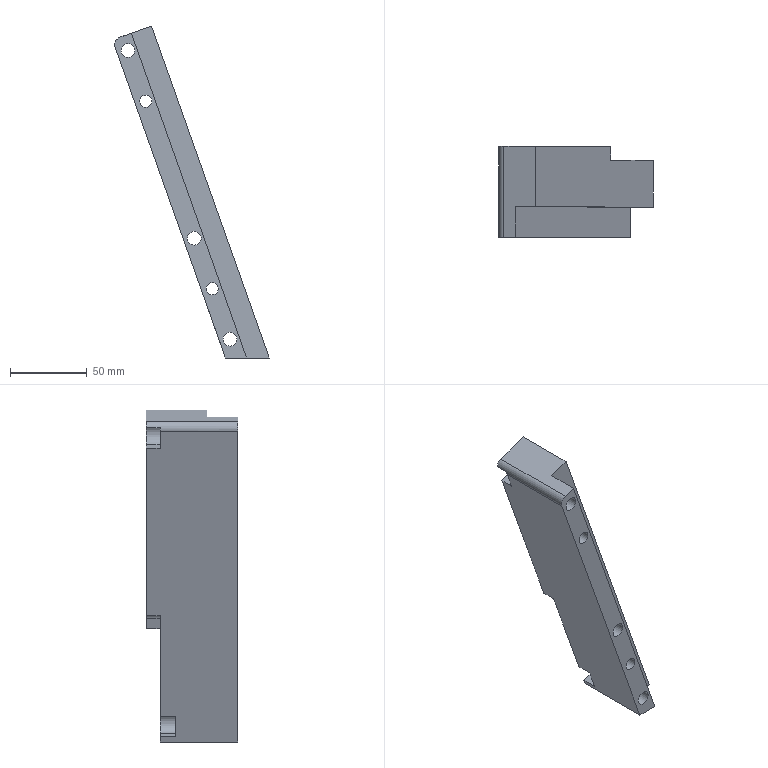Part | STEP file | SLIDE1-PLATE_id554_x_t | 1 solid | 27 faces | box 100.862 x 59.5 x 216.856 mm | volume 259316 mm3 | plane 18 | cylinder 9 | commonest cylinder face diameters 9 x3 14 x3 8 x2 10 x1
STEP:
#1=CARTESIAN_POINT('',(-1.05,-40.,-275.));
#2=VERTEX_POINT('',#1);
#3=CARTESIAN_POINT('',(13.802,-40.,-275.));
#4=VERTEX_POINT('',#3);
#5=CARTESIAN_POINT('',(-10.598,-40.,-275.));
#6=DIRECTION('',(1.,0.,0.));
#7=VECTOR('',#6,1.);
#8=LINE('',#5,#7);
#9=EDGE_CURVE('',#2,#4,#8,.T.);
#10=ORIENTED_EDGE('',*,*,#9,.T.);
#11=CARTESIAN_POINT('',(-62.991,-40.,-58.144));
#12=VERTEX_POINT('',#11);
#13=CARTESIAN_POINT('',(-62.991,-40.,-58.144));
#14=DIRECTION('',(0.3338,0.,-0.9426));
#15=VECTOR('',#14,1.);
#16=LINE('',#13,#15);
#17=EDGE_CURVE('',#12,#4,#16,.T.);
#18=ORIENTED_EDGE('',*,*,#17,.F.);
#19=CARTESIAN_POINT('',(-76.188,-40.,-62.818));
#20=VERTEX_POINT('',#19);
#21=CARTESIAN_POINT('',(11.277,-40.,-31.845));
#22=DIRECTION('',(-0.9426,0.,-0.3338));
#23=VECTOR('',#22,1.);
#24=LINE('',#21,#23);
#25=EDGE_CURVE('',#12,#20,#24,.T.);
#26=ORIENTED_EDGE('',*,*,#25,.T.);
#27=CARTESIAN_POINT('',(-76.188,-40.,-62.818));
#28=DIRECTION('',(0.3338,0.,-0.9426));
#29=VECTOR('',#28,1.);
#30=LINE('',#27,#29);
#31=EDGE_CURVE('',#20,#2,#30,.T.);
#32=ORIENTED_EDGE('',*,*,#31,.T.);
#33=EDGE_LOOP('',(#10,#18,#26,#32));
#34=FACE_OUTER_BOUND('',#33,.T.);
#35=CARTESIAN_POINT('',(-62.991,-40.,-58.144));
#36=DIRECTION('',(0.,1.,0.));
#37=DIRECTION('',(0.,0.,1.));
#38=AXIS2_PLACEMENT_3D('',#35,#36,#37);
#39=PLANE('',#38);
#40=ADVANCED_FACE('',(#34),#39,.F.);
#41=CARTESIAN_POINT('',(-1.05,-60.,-275.));
#42=VERTEX_POINT('',#41);
#43=CARTESIAN_POINT('',(-1.05,-0.5,-275.));
#44=DIRECTION('',(0.,1.,0.));
#45=VECTOR('',#44,1.);
#46=LINE('',#43,#45);
#47=EDGE_CURVE('',#42,#2,#46,.T.);
#48=ORIENTED_EDGE('',*,*,#47,.T.);
#49=ORIENTED_EDGE('',*,*,#31,.F.);
#50=CARTESIAN_POINT('',(-76.188,-60.,-62.818));
#51=VERTEX_POINT('',#50);
#52=CARTESIAN_POINT('',(-76.188,60.,-62.818));
#53=DIRECTION('',(0.,-1.,0.));
#54=VECTOR('',#53,1.);
#55=LINE('',#52,#54);
#56=EDGE_CURVE('',#20,#51,#55,.T.);
#57=ORIENTED_EDGE('',*,*,#56,.T.);
#58=CARTESIAN_POINT('',(-1.05,-60.,-275.));
#59=DIRECTION('',(-0.3338,0.,0.9426));
#60=VECTOR('',#59,1.);
#61=LINE('',#58,#60);
#62=EDGE_CURVE('',#42,#51,#61,.T.);
#63=ORIENTED_EDGE('',*,*,#62,.F.);
#64=EDGE_LOOP('',(#48,#49,#57,#63));
#65=FACE_OUTER_BOUND('',#64,.T.);
#66=CARTESIAN_POINT('',(-76.188,-40.,-62.818));
#67=DIRECTION('',(-0.9426,0.,-0.3338));
#68=DIRECTION('',(-0.3338,0.,0.9426));
#69=AXIS2_PLACEMENT_3D('',#66,#67,#68);
#70=PLANE('',#69);
#71=ADVANCED_FACE('',(#65),#70,.F.);
#72=CARTESIAN_POINT('',(-78.506,-60.,-69.747));
#73=VERTEX_POINT('',#72);
#74=CARTESIAN_POINT('',(-78.506,-60.,-74.247));
#75=DIRECTION('',(0.,1.,0.));
#76=DIRECTION('',(0.,0.,1.));
#77=AXIS2_PLACEMENT_3D('',#74,#75,#76);
#78=CIRCLE('',#77,4.5);
#79=EDGE_CURVE('',#73,#73,#78,.T.);
#80=ORIENTED_EDGE('',*,*,#79,.F.);
#81=EDGE_LOOP('',(#80));
#82=FACE_BOUND('',#81,.T.);
#83=CARTESIAN_POINT('',(-78.506,-9.5,-69.747));
#84=VERTEX_POINT('',#83);
#85=CARTESIAN_POINT('',(-78.506,-9.5,-74.247));
#86=DIRECTION('',(0.,-1.,0.));
#87=DIRECTION('',(0.,0.,1.));
#88=AXIS2_PLACEMENT_3D('',#85,#86,#87);
#89=CIRCLE('',#88,4.5);
#90=EDGE_CURVE('',#84,#84,#89,.T.);
#91=ORIENTED_EDGE('',*,*,#90,.F.);
#92=EDGE_LOOP('',(#91));
#93=FACE_BOUND('',#92,.T.);
#94=CARTESIAN_POINT('',(-78.506,-0.5,-74.247));
#95=DIRECTION('',(0.,1.,0.));
#96=DIRECTION('',(0.,0.,1.));
#97=AXIS2_PLACEMENT_3D('',#94,#95,#96);
#98=CYLINDRICAL_SURFACE('',#97,4.5);
#99=ADVANCED_FACE('',(#82,#93),#98,.F.);
#100=CARTESIAN_POINT('',(-80.842,-9.5,-67.648));
#101=VERTEX_POINT('',#100);
#102=CARTESIAN_POINT('',(-76.169,-9.5,-80.845));
#103=VERTEX_POINT('',#102);
#104=CARTESIAN_POINT('',(-78.506,-9.5,-74.247));
#105=DIRECTION('',(0.,1.,0.));
#106=DIRECTION('',(0.,0.,1.));
#107=AXIS2_PLACEMENT_3D('',#104,#105,#106);
#108=CIRCLE('',#107,7.);
#109=EDGE_CURVE('',#101,#103,#108,.T.);
#110=ORIENTED_EDGE('',*,*,#109,.F.);
#111=CARTESIAN_POINT('',(-80.842,-0.5,-67.648));
#112=VERTEX_POINT('',#111);
#113=CARTESIAN_POINT('',(-80.842,-0.5,-67.648));
#114=DIRECTION('',(0.,1.,0.));
#115=VECTOR('',#114,1.);
#116=LINE('',#113,#115);
#117=EDGE_CURVE('',#101,#112,#116,.T.);
#118=ORIENTED_EDGE('',*,*,#117,.T.);
#119=CARTESIAN_POINT('',(-76.169,-0.5,-80.845));
#120=VERTEX_POINT('',#119);
#121=CARTESIAN_POINT('',(-78.506,-0.5,-74.247));
#122=DIRECTION('',(0.,-1.,0.));
#123=DIRECTION('',(0.,0.,1.));
#124=AXIS2_PLACEMENT_3D('',#121,#122,#123);
#125=CIRCLE('',#124,7.);
#126=EDGE_CURVE('',#120,#112,#125,.T.);
#127=ORIENTED_EDGE('',*,*,#126,.F.);
#128=CARTESIAN_POINT('',(-76.169,-0.5,-80.845));
#129=DIRECTION('',(0.,-1.,0.));
#130=VECTOR('',#129,1.);
#131=LINE('',#128,#130);
#132=EDGE_CURVE('',#120,#103,#131,.T.);
#133=ORIENTED_EDGE('',*,*,#132,.T.);
#134=EDGE_LOOP('',(#110,#118,#127,#133));
#135=FACE_OUTER_BOUND('',#134,.T.);
#136=CARTESIAN_POINT('',(-78.506,-0.5,-74.247));
#137=DIRECTION('',(0.,1.,0.));
#138=DIRECTION('',(0.,0.,1.));
#139=AXIS2_PLACEMENT_3D('',#136,#137,#138);
#140=CYLINDRICAL_SURFACE('',#139,7.);
#141=ADVANCED_FACE('',(#135),#140,.F.);
#142=CARTESIAN_POINT('',(-87.047,-9.5,-69.846));
#143=VERTEX_POINT('',#142);
#144=CARTESIAN_POINT('',(-87.047,-9.5,-69.846));
#145=DIRECTION('',(0.9426,0.,0.3338));
#146=VECTOR('',#145,1.);
#147=LINE('',#144,#146);
#148=EDGE_CURVE('',#143,#101,#147,.T.);
#149=ORIENTED_EDGE('',*,*,#148,.F.);
#150=CARTESIAN_POINT('',(-87.047,-0.5,-69.846));
#151=VERTEX_POINT('',#150);
#152=CARTESIAN_POINT('',(-87.047,-0.5,-69.846));
#153=DIRECTION('',(0.,-1.,0.));
#154=VECTOR('',#153,1.);
#155=LINE('',#152,#154);
#156=EDGE_CURVE('',#151,#143,#155,.T.);
#157=ORIENTED_EDGE('',*,*,#156,.F.);
#158=CARTESIAN_POINT('',(-80.842,-0.5,-67.648));
#159=DIRECTION('',(-0.9426,0.,-0.3338));
#160=VECTOR('',#159,1.);
#161=LINE('',#158,#160);
#162=EDGE_CURVE('',#112,#151,#161,.T.);
#163=ORIENTED_EDGE('',*,*,#162,.F.);
#164=ORIENTED_EDGE('',*,*,#117,.F.);
#165=EDGE_LOOP('',(#149,#157,#163,#164));
#166=FACE_OUTER_BOUND('',#165,.T.);
#167=CARTESIAN_POINT('',(-94.861,-0.5,-72.613));
#168=DIRECTION('',(-0.3338,0.,0.9426));
#169=DIRECTION('',(0.9426,0.,0.3338));
#170=AXIS2_PLACEMENT_3D('',#167,#168,#169);
#171=PLANE('',#170);
#172=ADVANCED_FACE('',(#166),#171,.F.);
#173=CARTESIAN_POINT('',(-62.991,-0.5,-58.144));
#174=VERTEX_POINT('',#173);
#175=CARTESIAN_POINT('',(-62.991,-0.5,-58.144));
#176=DIRECTION('',(0.,-1.,0.));
#177=VECTOR('',#176,1.);
#178=LINE('',#175,#177);
#179=EDGE_CURVE('',#174,#12,#178,.T.);
#180=ORIENTED_EDGE('',*,*,#179,.F.);
#181=CARTESIAN_POINT('',(-83.729,-0.5,-65.488));
#182=VERTEX_POINT('',#181);
#183=CARTESIAN_POINT('',(-83.729,-0.5,-65.488));
#184=DIRECTION('',(0.9426,0.,0.3338));
#185=VECTOR('',#184,1.);
#186=LINE('',#183,#185);
#187=EDGE_CURVE('',#182,#174,#186,.T.);
#188=ORIENTED_EDGE('',*,*,#187,.F.);
#189=CARTESIAN_POINT('',(-83.729,-60.,-65.488));
#190=VERTEX_POINT('',#189);
#191=CARTESIAN_POINT('',(-83.729,-0.5,-65.488));
#192=DIRECTION('',(0.,1.,0.));
#193=VECTOR('',#192,1.);
#194=LINE('',#191,#193);
#195=EDGE_CURVE('',#190,#182,#194,.T.);
#196=ORIENTED_EDGE('',*,*,#195,.F.);
#197=CARTESIAN_POINT('',(-76.188,-60.,-62.818));
#198=DIRECTION('',(-0.9426,0.,-0.3338));
#199=VECTOR('',#198,1.);
#200=LINE('',#197,#199);
#201=EDGE_CURVE('',#51,#190,#200,.T.);
#202=ORIENTED_EDGE('',*,*,#201,.F.);
#203=ORIENTED_EDGE('',*,*,#56,.F.);
#204=ORIENTED_EDGE('',*,*,#25,.F.);
#205=EDGE_LOOP('',(#180,#188,#196,#202,#203,#204));
#206=FACE_OUTER_BOUND('',#205,.T.);
#207=CARTESIAN_POINT('',(11.277,60.,-31.845));
#208=DIRECTION('',(0.3338,0.,-0.9426));
#209=DIRECTION('',(-0.9426,0.,-0.3338));
#210=AXIS2_PLACEMENT_3D('',#207,#208,#209);
#211=PLANE('',#210);
#212=ADVANCED_FACE('',(#206),#211,.F.);
#213=CARTESIAN_POINT('',(-66.822,-60.,-103.239));
#214=VERTEX_POINT('',#213);
#215=CARTESIAN_POINT('',(-66.822,-60.,-107.239));
#216=DIRECTION('',(0.,1.,0.));
#217=DIRECTION('',(0.,0.,1.));
#218=AXIS2_PLACEMENT_3D('',#215,#216,#217);
#219=CIRCLE('',#218,4.);
#220=EDGE_CURVE('',#214,#214,#219,.T.);
#221=ORIENTED_EDGE('',*,*,#220,.F.);
#222=EDGE_LOOP('',(#221));
#223=FACE_BOUND('',#222,.T.);
#224=CARTESIAN_POINT('',(-66.822,-0.5,-103.239));
#225=VERTEX_POINT('',#224);
#226=CARTESIAN_POINT('',(-66.822,-0.5,-107.239));
#227=DIRECTION('',(0.,-1.,0.));
#228=DIRECTION('',(0.,0.,1.));
#229=AXIS2_PLACEMENT_3D('',#226,#227,#228);
#230=CIRCLE('',#229,4.);
#231=EDGE_CURVE('',#225,#225,#230,.T.);
#232=ORIENTED_EDGE('',*,*,#231,.F.);
#233=EDGE_LOOP('',(#232));
#234=FACE_BOUND('',#233,.T.);
#235=CARTESIAN_POINT('',(-66.822,-0.5,-107.239));
#236=DIRECTION('',(0.,1.,0.));
#237=DIRECTION('',(0.,0.,1.));
#238=AXIS2_PLACEMENT_3D('',#235,#236,#237);
#239=CYLINDRICAL_SURFACE('',#238,4.);
#240=ADVANCED_FACE('',(#223,#234),#239,.F.);
#241=CARTESIAN_POINT('',(-11.744,-60.,-258.275));
#242=VERTEX_POINT('',#241);
#243=CARTESIAN_POINT('',(-11.744,-60.,-262.775));
#244=DIRECTION('',(0.,1.,0.));
#245=DIRECTION('',(0.,0.,1.));
#246=AXIS2_PLACEMENT_3D('',#243,#244,#245);
#247=CIRCLE('',#246,4.5);
#248=EDGE_CURVE('',#242,#242,#247,.T.);
#249=ORIENTED_EDGE('',*,*,#248,.F.);
#250=EDGE_LOOP('',(#249));
#251=FACE_BOUND('',#250,.T.);
#252=CARTESIAN_POINT('',(-11.744,-19.5,-258.275));
#253=VERTEX_POINT('',#252);
#254=CARTESIAN_POINT('',(-11.744,-19.5,-262.775));
#255=DIRECTION('',(0.,-1.,0.));
#256=DIRECTION('',(0.,0.,1.));
#257=AXIS2_PLACEMENT_3D('',#254,#255,#256);
#258=CIRCLE('',#257,4.5);
#259=EDGE_CURVE('',#253,#253,#258,.T.);
#260=ORIENTED_EDGE('',*,*,#259,.F.);
#261=EDGE_LOOP('',(#260));
#262=FACE_BOUND('',#261,.T.);
#263=CARTESIAN_POINT('',(-11.744,-0.5,-262.775));
#264=DIRECTION('',(0.,1.,0.));
#265=DIRECTION('',(0.,0.,1.));
#266=AXIS2_PLACEMENT_3D('',#263,#264,#265);
#267=CYLINDRICAL_SURFACE('',#266,4.5);
#268=ADVANCED_FACE('',(#251,#262),#267,.F.);
#269=CARTESIAN_POINT('',(-37.447,-9.5,-190.192));
#270=VERTEX_POINT('',#269);
#271=CARTESIAN_POINT('',(-37.447,-0.5,-190.192));
#272=VERTEX_POINT('',#271);
#273=CARTESIAN_POINT('',(-37.447,-0.5,-190.192));
#274=DIRECTION('',(0.,1.,0.));
#275=VECTOR('',#274,1.);
#276=LINE('',#273,#275);
#277=EDGE_CURVE('',#270,#272,#276,.T.);
#278=ORIENTED_EDGE('',*,*,#277,.T.);
#279=CARTESIAN_POINT('',(-28.512,-0.5,-194.454));
#280=VERTEX_POINT('',#279);
#281=CARTESIAN_POINT('',(-35.111,-0.5,-196.79));
#282=DIRECTION('',(0.,-1.,0.));
#283=DIRECTION('',(0.,0.,1.));
#284=AXIS2_PLACEMENT_3D('',#281,#282,#283);
#285=CIRCLE('',#284,7.);
#286=EDGE_CURVE('',#280,#272,#285,.T.);
#287=ORIENTED_EDGE('',*,*,#286,.F.);
#288=CARTESIAN_POINT('',(-28.512,-9.5,-194.454));
#289=VERTEX_POINT('',#288);
#290=CARTESIAN_POINT('',(-28.512,-0.5,-194.454));
#291=DIRECTION('',(0.,-1.,0.));
#292=VECTOR('',#291,1.);
#293=LINE('',#290,#292);
#294=EDGE_CURVE('',#280,#289,#293,.T.);
#295=ORIENTED_EDGE('',*,*,#294,.T.);
#296=CARTESIAN_POINT('',(-35.111,-9.5,-196.79));
#297=DIRECTION('',(0.,1.,0.));
#298=DIRECTION('',(0.,0.,1.));
#299=AXIS2_PLACEMENT_3D('',#296,#297,#298);
#300=CIRCLE('',#299,7.);
#301=EDGE_CURVE('',#270,#289,#300,.T.);
#302=ORIENTED_EDGE('',*,*,#301,.F.);
#303=EDGE_LOOP('',(#278,#287,#295,#302));
#304=FACE_OUTER_BOUND('',#303,.T.);
#305=CARTESIAN_POINT('',(-35.111,-0.5,-196.79));
#306=DIRECTION('',(0.,1.,0.));
#307=DIRECTION('',(0.,0.,1.));
#308=AXIS2_PLACEMENT_3D('',#305,#306,#307);
#309=CYLINDRICAL_SURFACE('',#308,7.);
#310=ADVANCED_FACE('',(#304),#309,.F.);
#311=CARTESIAN_POINT('',(-26.175,-9.5,-201.052));
#312=VERTEX_POINT('',#311);
#313=CARTESIAN_POINT('',(-28.512,-9.5,-194.454));
#314=DIRECTION('',(0.3338,0.,-0.9426));
#315=VECTOR('',#314,1.);
#316=LINE('',#313,#315);
#317=EDGE_CURVE('',#289,#312,#316,.T.);
#318=ORIENTED_EDGE('',*,*,#317,.F.);
#319=ORIENTED_EDGE('',*,*,#294,.F.);
#320=CARTESIAN_POINT('',(-26.175,-0.5,-201.052));
#321=VERTEX_POINT('',#320);
#322=CARTESIAN_POINT('',(-26.175,-0.5,-201.052));
#323=DIRECTION('',(-0.3338,0.,0.9426));
#324=VECTOR('',#323,1.);
#325=LINE('',#322,#324);
#326=EDGE_CURVE('',#321,#280,#325,.T.);
#327=ORIENTED_EDGE('',*,*,#326,.F.);
#328=CARTESIAN_POINT('',(-26.175,-0.5,-201.052));
#329=DIRECTION('',(0.,-1.,0.));
#330=VECTOR('',#329,1.);
#331=LINE('',#328,#330);
#332=EDGE_CURVE('',#321,#312,#331,.T.);
#333=ORIENTED_EDGE('',*,*,#332,.T.);
#334=EDGE_LOOP('',(#318,#319,#327,#333));
#335=FACE_OUTER_BOUND('',#334,.T.);
#336=CARTESIAN_POINT('',(-28.512,-0.5,-194.454));
#337=DIRECTION('',(0.9426,0.,0.3338));
#338=DIRECTION('',(0.3338,0.,-0.9426));
#339=AXIS2_PLACEMENT_3D('',#336,#337,#338);
#340=PLANE('',#339);
#341=ADVANCED_FACE('',(#335),#340,.F.);
#342=CARTESIAN_POINT('',(-13.921,-9.5,-196.713));
#343=VERTEX_POINT('',#342);
#344=CARTESIAN_POINT('',(-26.175,-9.5,-201.052));
#345=DIRECTION('',(0.9426,0.,0.3338));
#346=VECTOR('',#345,1.);
#347=LINE('',#344,#346);
#348=EDGE_CURVE('',#312,#343,#347,.T.);
#349=ORIENTED_EDGE('',*,*,#348,.F.);
#350=ORIENTED_EDGE('',*,*,#332,.F.);
#351=CARTESIAN_POINT('',(-13.921,-0.5,-196.713));
#352=VERTEX_POINT('',#351);
#353=CARTESIAN_POINT('',(-13.921,-0.5,-196.713));
#354=DIRECTION('',(-0.9426,0.,-0.3338));
#355=VECTOR('',#354,1.);
#356=LINE('',#353,#355);
#357=EDGE_CURVE('',#352,#321,#356,.T.);
#358=ORIENTED_EDGE('',*,*,#357,.F.);
#359=CARTESIAN_POINT('',(-13.921,-0.5,-196.713));
#360=DIRECTION('',(0.,1.,0.));
#361=VECTOR('',#360,1.);
#362=LINE('',#359,#361);
#363=EDGE_CURVE('',#343,#352,#362,.T.);
#364=ORIENTED_EDGE('',*,*,#363,.F.);
#365=EDGE_LOOP('',(#349,#350,#358,#364));
#366=FACE_OUTER_BOUND('',#365,.T.);
#367=CARTESIAN_POINT('',(-26.175,-0.5,-201.052));
#368=DIRECTION('',(-0.3338,0.,0.9426));
#369=DIRECTION('',(0.9426,0.,0.3338));
#370=AXIS2_PLACEMENT_3D('',#367,#368,#369);
#371=PLANE('',#370);
#372=ADVANCED_FACE('',(#366),#371,.F.);
#373=CARTESIAN_POINT('',(13.802,-9.5,-275.));
#374=VERTEX_POINT('',#373);
#375=CARTESIAN_POINT('',(13.802,-0.5,-275.));
#376=DIRECTION('',(0.,1.,0.));
#377=VECTOR('',#376,1.);
#378=LINE('',#375,#377);
#379=EDGE_CURVE('',#4,#374,#378,.T.);
#380=ORIENTED_EDGE('',*,*,#379,.T.);
#381=CARTESIAN_POINT('',(-13.921,-9.5,-196.713));
#382=DIRECTION('',(0.3338,0.,-0.9426));
#383=VECTOR('',#382,1.);
#384=LINE('',#381,#383);
#385=EDGE_CURVE('',#343,#374,#384,.T.);
#386=ORIENTED_EDGE('',*,*,#385,.F.);
#387=ORIENTED_EDGE('',*,*,#363,.T.);
#388=CARTESIAN_POINT('',(-62.991,-0.5,-58.144));
#389=DIRECTION('',(0.3338,0.,-0.9426));
#390=VECTOR('',#389,1.);
#391=LINE('',#388,#390);
#392=EDGE_CURVE('',#174,#352,#391,.T.);
#393=ORIENTED_EDGE('',*,*,#392,.F.);
#394=ORIENTED_EDGE('',*,*,#179,.T.);
#395=ORIENTED_EDGE('',*,*,#17,.T.);
#396=EDGE_LOOP('',(#380,#386,#387,#393,#394,#395));
#397=FACE_OUTER_BOUND('',#396,.T.);
#398=CARTESIAN_POINT('',(-62.991,-0.5,-58.144));
#399=DIRECTION('',(0.9426,0.,0.3338));
#400=DIRECTION('',(0.3338,0.,-0.9426));
#401=AXIS2_PLACEMENT_3D('',#398,#399,#400);
#402=PLANE('',#401);
#403=ADVANCED_FACE('',(#397),#402,.T.);
#404=CARTESIAN_POINT('',(-14.081,-19.5,-256.177));
#405=VERTEX_POINT('',#404);
#406=CARTESIAN_POINT('',(-9.407,-19.5,-269.374));
#407=VERTEX_POINT('',#406);
#408=CARTESIAN_POINT('',(-11.744,-19.5,-262.775));
#409=DIRECTION('',(0.,1.,0.));
#410=DIRECTION('',(0.,0.,1.));
#411=AXIS2_PLACEMENT_3D('',#408,#409,#410);
#412=CIRCLE('',#411,7.);
#413=EDGE_CURVE('',#405,#407,#412,.T.);
#414=ORIENTED_EDGE('',*,*,#413,.F.);
#415=CARTESIAN_POINT('',(-14.081,-9.5,-256.177));
#416=VERTEX_POINT('',#415);
#417=CARTESIAN_POINT('',(-14.081,-0.5,-256.177));
#418=DIRECTION('',(0.,1.,0.));
#419=VECTOR('',#418,1.);
#420=LINE('',#417,#419);
#421=EDGE_CURVE('',#405,#416,#420,.T.);
#422=ORIENTED_EDGE('',*,*,#421,.T.);
#423=CARTESIAN_POINT('',(-9.407,-9.5,-269.374));
#424=VERTEX_POINT('',#423);
#425=CARTESIAN_POINT('',(-11.744,-9.5,-262.775));
#426=DIRECTION('',(0.,-1.,0.));
#427=DIRECTION('',(0.,0.,1.));
#428=AXIS2_PLACEMENT_3D('',#425,#426,#427);
#429=CIRCLE('',#428,7.);
#430=EDGE_CURVE('',#424,#416,#429,.T.);
#431=ORIENTED_EDGE('',*,*,#430,.F.);
#432=CARTESIAN_POINT('',(-9.407,-0.5,-269.374));
#433=DIRECTION('',(0.,-1.,0.));
#434=VECTOR('',#433,1.);
#435=LINE('',#432,#434);
#436=EDGE_CURVE('',#424,#407,#435,.T.);
#437=ORIENTED_EDGE('',*,*,#436,.T.);
#438=EDGE_LOOP('',(#414,#422,#431,#437));
#439=FACE_OUTER_BOUND('',#438,.T.);
#440=CARTESIAN_POINT('',(-11.744,-0.5,-262.775));
#441=DIRECTION('',(0.,1.,0.));
#442=DIRECTION('',(0.,0.,1.));
#443=AXIS2_PLACEMENT_3D('',#440,#441,#442);
#444=CYLINDRICAL_SURFACE('',#443,7.);
#445=ADVANCED_FACE('',(#439),#444,.F.);
#446=CARTESIAN_POINT('',(-23.427,-60.,-225.783));
#447=VERTEX_POINT('',#446);
#448=CARTESIAN_POINT('',(-23.427,-60.,-229.783));
#449=DIRECTION('',(0.,1.,0.));
#450=DIRECTION('',(0.,0.,1.));
#451=AXIS2_PLACEMENT_3D('',#448,#449,#450);
#452=CIRCLE('',#451,4.);
#453=EDGE_CURVE('',#447,#447,#452,.T.);
#454=ORIENTED_EDGE('',*,*,#453,.F.);
#455=EDGE_LOOP('',(#454));
#456=FACE_BOUND('',#455,.T.);
#457=CARTESIAN_POINT('',(-23.427,-9.5,-225.783));
#458=VERTEX_POINT('',#457);
#459=CARTESIAN_POINT('',(-23.427,-9.5,-229.783));
#460=DIRECTION('',(0.,-1.,0.));
#461=DIRECTION('',(0.,0.,1.));
#462=AXIS2_PLACEMENT_3D('',#459,#460,#461);
#463=CIRCLE('',#462,4.);
#464=EDGE_CURVE('',#458,#458,#463,.T.);
#465=ORIENTED_EDGE('',*,*,#464,.F.);
#466=EDGE_LOOP('',(#465));
#467=FACE_BOUND('',#466,.T.);
#468=CARTESIAN_POINT('',(-23.427,-0.5,-229.783));
#469=DIRECTION('',(0.,1.,0.));
#470=DIRECTION('',(0.,0.,1.));
#471=AXIS2_PLACEMENT_3D('',#468,#469,#470);
#472=CYLINDRICAL_SURFACE('',#471,4.);
#473=ADVANCED_FACE('',(#456,#467),#472,.F.);
#474=CARTESIAN_POINT('',(-35.111,-60.,-192.29));
#475=VERTEX_POINT('',#474);
#476=CARTESIAN_POINT('',(-35.111,-60.,-196.79));
#477=DIRECTION('',(0.,1.,0.));
#478=DIRECTION('',(0.,0.,1.));
#479=AXIS2_PLACEMENT_3D('',#476,#477,#478);
#480=CIRCLE('',#479,4.5);
#481=EDGE_CURVE('',#475,#475,#480,.T.);
#482=ORIENTED_EDGE('',*,*,#481,.F.);
#483=EDGE_LOOP('',(#482));
#484=FACE_BOUND('',#483,.T.);
#485=CARTESIAN_POINT('',(-35.111,-9.5,-192.29));
#486=VERTEX_POINT('',#485);
#487=CARTESIAN_POINT('',(-35.111,-9.5,-196.79));
#488=DIRECTION('',(0.,-1.,0.));
#489=DIRECTION('',(0.,0.,1.));
#490=AXIS2_PLACEMENT_3D('',#487,#488,#489);
#491=CIRCLE('',#490,4.5);
#492=EDGE_CURVE('',#486,#486,#491,.T.);
#493=ORIENTED_EDGE('',*,*,#492,.F.);
#494=EDGE_LOOP('',(#493));
#495=FACE_BOUND('',#494,.T.);
#496=CARTESIAN_POINT('',(-35.111,-0.5,-196.79));
#497=DIRECTION('',(0.,1.,0.));
#498=DIRECTION('',(0.,0.,1.));
#499=AXIS2_PLACEMENT_3D('',#496,#497,#498);
#500=CYLINDRICAL_SURFACE('',#499,4.5);
#501=ADVANCED_FACE('',(#484,#495),#500,.F.);
#502=ORIENTED_EDGE('',*,*,#9,.F.);
#503=ORIENTED_EDGE('',*,*,#47,.F.);
#504=CARTESIAN_POINT('',(-14.841,-60.,-275.));
#505=VERTEX_POINT('',#504);
#506=CARTESIAN_POINT('',(-70.532,-60.,-275.));
#507=DIRECTION('',(1.,0.,0.));
#508=VECTOR('',#507,1.);
#509=LINE('',#506,#508);
#510=EDGE_CURVE('',#505,#42,#509,.T.);
#511=ORIENTED_EDGE('',*,*,#510,.F.);
#512=CARTESIAN_POINT('',(-14.841,-9.5,-275.));
#513=VERTEX_POINT('',#512);
#514=CARTESIAN_POINT('',(-14.841,-0.5,-275.));
#515=DIRECTION('',(0.,-1.,0.));
#516=VECTOR('',#515,1.);
#517=LINE('',#514,#516);
#518=EDGE_CURVE('',#513,#505,#517,.T.);
#519=ORIENTED_EDGE('',*,*,#518,.F.);
#520=CARTESIAN_POINT('',(11.277,-9.5,-275.));
#521=DIRECTION('',(-1.,0.,0.));
#522=VECTOR('',#521,1.);
#523=LINE('',#520,#522);
#524=EDGE_CURVE('',#374,#513,#523,.T.);
#525=ORIENTED_EDGE('',*,*,#524,.F.);
#526=ORIENTED_EDGE('',*,*,#379,.F.);
#527=EDGE_LOOP('',(#502,#503,#511,#519,#525,#526));
#528=FACE_OUTER_BOUND('',#527,.T.);
#529=CARTESIAN_POINT('',(-10.598,-0.5,-275.));
#530=DIRECTION('',(0.,0.,1.));
#531=DIRECTION('',(1.,0.,0.));
#532=AXIS2_PLACEMENT_3D('',#529,#530,#531);
#533=PLANE('',#532);
#534=ADVANCED_FACE('',(#528),#533,.F.);
#535=ORIENTED_EDGE('',*,*,#248,.T.);
#536=EDGE_LOOP('',(#535));
#537=FACE_BOUND('',#536,.T.);
#538=ORIENTED_EDGE('',*,*,#453,.T.);
#539=EDGE_LOOP('',(#538));
#540=FACE_BOUND('',#539,.T.);
#541=ORIENTED_EDGE('',*,*,#481,.T.);
#542=EDGE_LOOP('',(#541));
#543=FACE_BOUND('',#542,.T.);
#544=ORIENTED_EDGE('',*,*,#220,.T.);
#545=EDGE_LOOP('',(#544));
#546=FACE_BOUND('',#545,.T.);
#547=ORIENTED_EDGE('',*,*,#79,.T.);
#548=EDGE_LOOP('',(#547));
#549=FACE_BOUND('',#548,.T.);
#550=ORIENTED_EDGE('',*,*,#510,.T.);
#551=ORIENTED_EDGE('',*,*,#62,.T.);
#552=ORIENTED_EDGE('',*,*,#201,.T.);
#553=CARTESIAN_POINT('',(-86.773,-60.,-71.87));
#554=VERTEX_POINT('',#553);
#555=CARTESIAN_POINT('',(-82.06,-60.,-70.201));
#556=DIRECTION('',(0.,1.,0.));
#557=DIRECTION('',(0.,0.,-1.));
#558=AXIS2_PLACEMENT_3D('',#555,#556,#557);
#559=CIRCLE('',#558,5.);
#560=EDGE_CURVE('',#554,#190,#559,.T.);
#561=ORIENTED_EDGE('',*,*,#560,.F.);
#562=CARTESIAN_POINT('',(-86.773,-60.,-71.87));
#563=DIRECTION('',(-0.3338,0.,0.9426));
#564=VECTOR('',#563,1.);
#565=LINE('',#562,#564);
#566=EDGE_CURVE('',#505,#554,#565,.T.);
#567=ORIENTED_EDGE('',*,*,#566,.F.);
#568=EDGE_LOOP('',(#550,#551,#552,#561,#567));
#569=FACE_BOUND('',#568,.T.);
#570=CARTESIAN_POINT('',(-70.532,-60.,-60.815));
#571=DIRECTION('',(0.,-1.,0.));
#572=DIRECTION('',(0.,0.,-1.));
#573=AXIS2_PLACEMENT_3D('',#570,#571,#572);
#574=PLANE('',#573);
#575=ADVANCED_FACE('',(#537,#540,#543,#546,#549,#569),#574,.T.);
#576=ORIENTED_EDGE('',*,*,#156,.T.);
#577=CARTESIAN_POINT('',(-86.773,-9.5,-71.87));
#578=VERTEX_POINT('',#577);
#579=CARTESIAN_POINT('',(-82.06,-9.5,-70.201));
#580=DIRECTION('',(0.,1.,0.));
#581=DIRECTION('',(0.,0.,-1.));
#582=AXIS2_PLACEMENT_3D('',#579,#580,#581);
#583=CIRCLE('',#582,5.);
#584=EDGE_CURVE('',#578,#143,#583,.T.);
#585=ORIENTED_EDGE('',*,*,#584,.F.);
#586=CARTESIAN_POINT('',(-86.773,-0.5,-71.87));
#587=DIRECTION('',(0.,1.,0.));
#588=VECTOR('',#587,1.);
#589=LINE('',#586,#588);
#590=EDGE_CURVE('',#554,#578,#589,.T.);
#591=ORIENTED_EDGE('',*,*,#590,.F.);
#592=ORIENTED_EDGE('',*,*,#560,.T.);
#593=ORIENTED_EDGE('',*,*,#195,.T.);
#594=CARTESIAN_POINT('',(-82.06,-0.5,-70.201));
#595=DIRECTION('',(0.,1.,0.));
#596=DIRECTION('',(0.,0.,-1.));
#597=AXIS2_PLACEMENT_3D('',#594,#595,#596);
#598=CIRCLE('',#597,5.);
#599=EDGE_CURVE('',#151,#182,#598,.T.);
#600=ORIENTED_EDGE('',*,*,#599,.F.);
#601=EDGE_LOOP('',(#576,#585,#591,#592,#593,#600));
#602=FACE_OUTER_BOUND('',#601,.T.);
#603=CARTESIAN_POINT('',(-82.06,-0.5,-70.201));
#604=DIRECTION('',(0.,-1.,0.));
#605=DIRECTION('',(0.,0.,-1.));
#606=AXIS2_PLACEMENT_3D('',#603,#604,#605);
#607=CYLINDRICAL_SURFACE('',#606,5.);
#608=ADVANCED_FACE('',(#602),#607,.T.);
#609=ORIENTED_EDGE('',*,*,#90,.T.);
#610=EDGE_LOOP('',(#609));
#611=FACE_BOUND('',#610,.T.);
#612=CARTESIAN_POINT('',(-82.767,-9.5,-83.182));
#613=VERTEX_POINT('',#612);
#614=CARTESIAN_POINT('',(-86.773,-9.5,-71.87));
#615=DIRECTION('',(0.3338,0.,-0.9426));
#616=VECTOR('',#615,1.);
#617=LINE('',#614,#616);
#618=EDGE_CURVE('',#578,#613,#617,.T.);
#619=ORIENTED_EDGE('',*,*,#618,.F.);
#620=ORIENTED_EDGE('',*,*,#584,.T.);
#621=ORIENTED_EDGE('',*,*,#148,.T.);
#622=ORIENTED_EDGE('',*,*,#109,.T.);
#623=CARTESIAN_POINT('',(-76.169,-9.5,-80.845));
#624=DIRECTION('',(-0.9426,0.,-0.3338));
#625=VECTOR('',#624,1.);
#626=LINE('',#623,#625);
#627=EDGE_CURVE('',#103,#613,#626,.T.);
#628=ORIENTED_EDGE('',*,*,#627,.T.);
#629=EDGE_LOOP('',(#619,#620,#621,#622,#628));
#630=FACE_BOUND('',#629,.T.);
#631=CARTESIAN_POINT('',(11.277,-9.5,-31.845));
#632=DIRECTION('',(0.,1.,0.));
#633=DIRECTION('',(0.,0.,1.));
#634=AXIS2_PLACEMENT_3D('',#631,#632,#633);
#635=PLANE('',#634);
#636=ADVANCED_FACE('',(#611,#630),#635,.T.);
#637=ORIENTED_EDGE('',*,*,#627,.F.);
#638=ORIENTED_EDGE('',*,*,#132,.F.);
#639=CARTESIAN_POINT('',(-82.767,-0.5,-83.182));
#640=VERTEX_POINT('',#639);
#641=CARTESIAN_POINT('',(-82.767,-0.5,-83.182));
#642=DIRECTION('',(0.9426,0.,0.3338));
#643=VECTOR('',#642,1.);
#644=LINE('',#641,#643);
#645=EDGE_CURVE('',#640,#120,#644,.T.);
#646=ORIENTED_EDGE('',*,*,#645,.F.);
#647=CARTESIAN_POINT('',(-82.767,-0.5,-83.182));
#648=DIRECTION('',(0.,1.,0.));
#649=VECTOR('',#648,1.);
#650=LINE('',#647,#649);
#651=EDGE_CURVE('',#613,#640,#650,.T.);
#652=ORIENTED_EDGE('',*,*,#651,.F.);
#653=EDGE_LOOP('',(#637,#638,#646,#652));
#654=FACE_OUTER_BOUND('',#653,.T.);
#655=CARTESIAN_POINT('',(-76.169,-0.5,-80.845));
#656=DIRECTION('',(0.3338,0.,-0.9426));
#657=DIRECTION('',(-0.9426,0.,-0.3338));
#658=AXIS2_PLACEMENT_3D('',#655,#656,#657);
#659=PLANE('',#658);
#660=ADVANCED_FACE('',(#654),#659,.F.);
#661=ORIENTED_EDGE('',*,*,#231,.T.);
#662=EDGE_LOOP('',(#661));
#663=FACE_BOUND('',#662,.T.);
#664=ORIENTED_EDGE('',*,*,#357,.T.);
#665=ORIENTED_EDGE('',*,*,#326,.T.);
#666=ORIENTED_EDGE('',*,*,#286,.T.);
#667=CARTESIAN_POINT('',(-44.046,-0.5,-192.528));
#668=VERTEX_POINT('',#667);
#669=CARTESIAN_POINT('',(-50.644,-0.5,-194.865));
#670=DIRECTION('',(-0.9426,0.,-0.3338));
#671=VECTOR('',#670,1.);
#672=LINE('',#669,#671);
#673=EDGE_CURVE('',#272,#668,#672,.T.);
#674=ORIENTED_EDGE('',*,*,#673,.T.);
#675=CARTESIAN_POINT('',(-86.773,-0.5,-71.87));
#676=DIRECTION('',(0.3338,0.,-0.9426));
#677=VECTOR('',#676,1.);
#678=LINE('',#675,#677);
#679=EDGE_CURVE('',#640,#668,#678,.T.);
#680=ORIENTED_EDGE('',*,*,#679,.F.);
#681=ORIENTED_EDGE('',*,*,#645,.T.);
#682=ORIENTED_EDGE('',*,*,#126,.T.);
#683=ORIENTED_EDGE('',*,*,#162,.T.);
#684=ORIENTED_EDGE('',*,*,#599,.T.);
#685=ORIENTED_EDGE('',*,*,#187,.T.);
#686=ORIENTED_EDGE('',*,*,#392,.T.);
#687=EDGE_LOOP('',(#664,#665,#666,#674,#680,#681,#682,#683,#684,#685,#686));
#688=FACE_BOUND('',#687,.T.);
#689=CARTESIAN_POINT('',(-84.671,-0.5,-65.822));
#690=DIRECTION('',(0.,1.,0.));
#691=DIRECTION('',(0.,0.,1.));
#692=AXIS2_PLACEMENT_3D('',#689,#690,#691);
#693=PLANE('',#692);
#694=ADVANCED_FACE('',(#663,#688),#693,.T.);
#695=CARTESIAN_POINT('',(-44.046,-9.5,-192.528));
#696=VERTEX_POINT('',#695);
#697=CARTESIAN_POINT('',(-44.046,-9.5,-192.528));
#698=DIRECTION('',(0.9426,0.,0.3338));
#699=VECTOR('',#698,1.);
#700=LINE('',#697,#699);
#701=EDGE_CURVE('',#696,#270,#700,.T.);
#702=ORIENTED_EDGE('',*,*,#701,.F.);
#703=CARTESIAN_POINT('',(-44.046,-0.5,-192.528));
#704=DIRECTION('',(0.,-1.,0.));
#705=VECTOR('',#704,1.);
#706=LINE('',#703,#705);
#707=EDGE_CURVE('',#668,#696,#706,.T.);
#708=ORIENTED_EDGE('',*,*,#707,.F.);
#709=ORIENTED_EDGE('',*,*,#673,.F.);
#710=ORIENTED_EDGE('',*,*,#277,.F.);
#711=EDGE_LOOP('',(#702,#708,#709,#710));
#712=FACE_OUTER_BOUND('',#711,.T.);
#713=CARTESIAN_POINT('',(-50.644,-0.5,-194.865));
#714=DIRECTION('',(-0.3338,0.,0.9426));
#715=DIRECTION('',(0.9426,0.,0.3338));
#716=AXIS2_PLACEMENT_3D('',#713,#714,#715);
#717=PLANE('',#716);
#718=ADVANCED_FACE('',(#712),#717,.F.);
#719=CARTESIAN_POINT('',(-20.679,-19.5,-258.513));
#720=VERTEX_POINT('',#719);
#721=CARTESIAN_POINT('',(-20.679,-19.5,-258.513));
#722=DIRECTION('',(0.9426,0.,0.3338));
#723=VECTOR('',#722,1.);
#724=LINE('',#721,#723);
#725=EDGE_CURVE('',#720,#405,#724,.T.);
#726=ORIENTED_EDGE('',*,*,#725,.F.);
#727=CARTESIAN_POINT('',(-20.679,-9.5,-258.513));
#728=VERTEX_POINT('',#727);
#729=CARTESIAN_POINT('',(-20.679,-0.5,-258.513));
#730=DIRECTION('',(0.,-1.,0.));
#731=VECTOR('',#730,1.);
#732=LINE('',#729,#731);
#733=EDGE_CURVE('',#728,#720,#732,.T.);
#734=ORIENTED_EDGE('',*,*,#733,.F.);
#735=CARTESIAN_POINT('',(-14.081,-9.5,-256.177));
#736=DIRECTION('',(-0.9426,0.,-0.3338));
#737=VECTOR('',#736,1.);
#738=LINE('',#735,#737);
#739=EDGE_CURVE('',#416,#728,#738,.T.);
#740=ORIENTED_EDGE('',*,*,#739,.F.);
#741=ORIENTED_EDGE('',*,*,#421,.F.);
#742=EDGE_LOOP('',(#726,#734,#740,#741));
#743=FACE_OUTER_BOUND('',#742,.T.);
#744=CARTESIAN_POINT('',(-31.655,-0.5,-262.4));
#745=DIRECTION('',(-0.3338,0.,0.9426));
#746=DIRECTION('',(0.9426,0.,0.3338));
#747=AXIS2_PLACEMENT_3D('',#744,#745,#746);
#748=PLANE('',#747);
#749=ADVANCED_FACE('',(#743),#748,.F.);
#750=ORIENTED_EDGE('',*,*,#259,.T.);
#751=EDGE_LOOP('',(#750));
#752=FACE_BOUND('',#751,.T.);
#753=CARTESIAN_POINT('',(-16.006,-19.5,-271.71));
#754=VERTEX_POINT('',#753);
#755=CARTESIAN_POINT('',(-9.407,-19.5,-269.374));
#756=DIRECTION('',(-0.9426,0.,-0.3338));
#757=VECTOR('',#756,1.);
#758=LINE('',#755,#757);
#759=EDGE_CURVE('',#407,#754,#758,.T.);
#760=ORIENTED_EDGE('',*,*,#759,.T.);
#761=CARTESIAN_POINT('',(-86.773,-19.5,-71.87));
#762=DIRECTION('',(0.3338,0.,-0.9426));
#763=VECTOR('',#762,1.);
#764=LINE('',#761,#763);
#765=EDGE_CURVE('',#720,#754,#764,.T.);
#766=ORIENTED_EDGE('',*,*,#765,.F.);
#767=ORIENTED_EDGE('',*,*,#725,.T.);
#768=ORIENTED_EDGE('',*,*,#413,.T.);
#769=EDGE_LOOP('',(#760,#766,#767,#768));
#770=FACE_BOUND('',#769,.T.);
#771=CARTESIAN_POINT('',(11.277,-19.5,-31.845));
#772=DIRECTION('',(0.,1.,0.));
#773=DIRECTION('',(0.,0.,1.));
#774=AXIS2_PLACEMENT_3D('',#771,#772,#773);
#775=PLANE('',#774);
#776=ADVANCED_FACE('',(#752,#770),#775,.T.);
#777=ORIENTED_EDGE('',*,*,#759,.F.);
#778=ORIENTED_EDGE('',*,*,#436,.F.);
#779=CARTESIAN_POINT('',(-16.006,-9.5,-271.71));
#780=VERTEX_POINT('',#779);
#781=CARTESIAN_POINT('',(-16.006,-9.5,-271.71));
#782=DIRECTION('',(0.9426,0.,0.3338));
#783=VECTOR('',#782,1.);
#784=LINE('',#781,#783);
#785=EDGE_CURVE('',#780,#424,#784,.T.);
#786=ORIENTED_EDGE('',*,*,#785,.F.);
#787=CARTESIAN_POINT('',(-16.006,-0.5,-271.71));
#788=DIRECTION('',(0.,1.,0.));
#789=VECTOR('',#788,1.);
#790=LINE('',#787,#789);
#791=EDGE_CURVE('',#754,#780,#790,.T.);
#792=ORIENTED_EDGE('',*,*,#791,.F.);
#793=EDGE_LOOP('',(#777,#778,#786,#792));
#794=FACE_OUTER_BOUND('',#793,.T.);
#795=CARTESIAN_POINT('',(-9.407,-0.5,-269.374));
#796=DIRECTION('',(0.3338,0.,-0.9426));
#797=DIRECTION('',(-0.9426,0.,-0.3338));
#798=AXIS2_PLACEMENT_3D('',#795,#796,#797);
#799=PLANE('',#798);
#800=ADVANCED_FACE('',(#794),#799,.F.);
#801=ORIENTED_EDGE('',*,*,#492,.T.);
#802=EDGE_LOOP('',(#801));
#803=FACE_BOUND('',#802,.T.);
#804=ORIENTED_EDGE('',*,*,#464,.T.);
#805=EDGE_LOOP('',(#804));
#806=FACE_BOUND('',#805,.T.);
#807=ORIENTED_EDGE('',*,*,#739,.T.);
#808=CARTESIAN_POINT('',(-86.773,-9.5,-71.87));
#809=DIRECTION('',(0.3338,0.,-0.9426));
#810=VECTOR('',#809,1.);
#811=LINE('',#808,#810);
#812=EDGE_CURVE('',#696,#728,#811,.T.);
#813=ORIENTED_EDGE('',*,*,#812,.F.);
#814=ORIENTED_EDGE('',*,*,#701,.T.);
#815=ORIENTED_EDGE('',*,*,#301,.T.);
#816=ORIENTED_EDGE('',*,*,#317,.T.);
#817=ORIENTED_EDGE('',*,*,#348,.T.);
#818=ORIENTED_EDGE('',*,*,#385,.T.);
#819=ORIENTED_EDGE('',*,*,#524,.T.);
#820=CARTESIAN_POINT('',(-86.773,-9.5,-71.87));
#821=DIRECTION('',(0.3338,0.,-0.9426));
#822=VECTOR('',#821,1.);
#823=LINE('',#820,#822);
#824=EDGE_CURVE('',#780,#513,#823,.T.);
#825=ORIENTED_EDGE('',*,*,#824,.F.);
#826=ORIENTED_EDGE('',*,*,#785,.T.);
#827=ORIENTED_EDGE('',*,*,#430,.T.);
#828=EDGE_LOOP('',(#807,#813,#814,#815,#816,#817,#818,#819,#825,#826,#827));
#829=FACE_BOUND('',#828,.T.);
#830=CARTESIAN_POINT('',(11.277,-9.5,-31.845));
#831=DIRECTION('',(0.,1.,0.));
#832=DIRECTION('',(0.,0.,1.));
#833=AXIS2_PLACEMENT_3D('',#830,#831,#832);
#834=PLANE('',#833);
#835=ADVANCED_FACE('',(#803,#806,#829),#834,.T.);
#836=ORIENTED_EDGE('',*,*,#791,.T.);
#837=ORIENTED_EDGE('',*,*,#824,.T.);
#838=ORIENTED_EDGE('',*,*,#518,.T.);
#839=ORIENTED_EDGE('',*,*,#566,.T.);
#840=ORIENTED_EDGE('',*,*,#590,.T.);
#841=ORIENTED_EDGE('',*,*,#618,.T.);
#842=ORIENTED_EDGE('',*,*,#651,.T.);
#843=ORIENTED_EDGE('',*,*,#679,.T.);
#844=ORIENTED_EDGE('',*,*,#707,.T.);
#845=ORIENTED_EDGE('',*,*,#812,.T.);
#846=ORIENTED_EDGE('',*,*,#733,.T.);
#847=ORIENTED_EDGE('',*,*,#765,.T.);
#848=EDGE_LOOP('',(#836,#837,#838,#839,#840,#841,#842,#843,#844,#845,#846,#847));
#849=FACE_OUTER_BOUND('',#848,.T.);
#850=CARTESIAN_POINT('',(-86.773,-0.5,-71.87));
#851=DIRECTION('',(-0.9426,0.,-0.3338));
#852=DIRECTION('',(-0.3338,0.,0.9426));
#853=AXIS2_PLACEMENT_3D('',#850,#851,#852);
#854=PLANE('',#853);
#855=ADVANCED_FACE('',(#849),#854,.T.);
#856=CLOSED_SHELL('',(#40,#71,#99,#141,#172,#212,#240,#268,#310,#341,#372,#403,#445,#473,#501,#534,#575,#608,#636,#660,#694,#718,#749,#776,#800,#835,#855));
#857=MANIFOLD_SOLID_BREP('',#856);
#858=(LENGTH_UNIT()NAMED_UNIT(*)SI_UNIT(.MILLI.,.METRE.));
#859=UNCERTAINTY_MEASURE_WITH_UNIT(LENGTH_MEASURE(0.00004123),#858,'','');
#860=(NAMED_UNIT(*)PLANE_ANGLE_UNIT()SI_UNIT($,.RADIAN.));
#861=PLANE_ANGLE_MEASURE_WITH_UNIT(PLANE_ANGLE_MEASURE(0.01745),#860);
#862=DIMENSIONAL_EXPONENTS(0.,0.,0.,0.,0.,0.,0.);
#863=(CONVERSION_BASED_UNIT('DEGREE',#861)NAMED_UNIT(#862)PLANE_ANGLE_UNIT());
#864=(NAMED_UNIT(*)SI_UNIT($,.STERADIAN.)SOLID_ANGLE_UNIT());
#865=(GEOMETRIC_REPRESENTATION_CONTEXT(3)GLOBAL_UNCERTAINTY_ASSIGNED_CONTEXT((#859))GLOBAL_UNIT_ASSIGNED_CONTEXT((#858,#863,#864))REPRESENTATION_CONTEXT('',''));
#866=ADVANCED_BREP_SHAPE_REPRESENTATION('',(#857),#865);